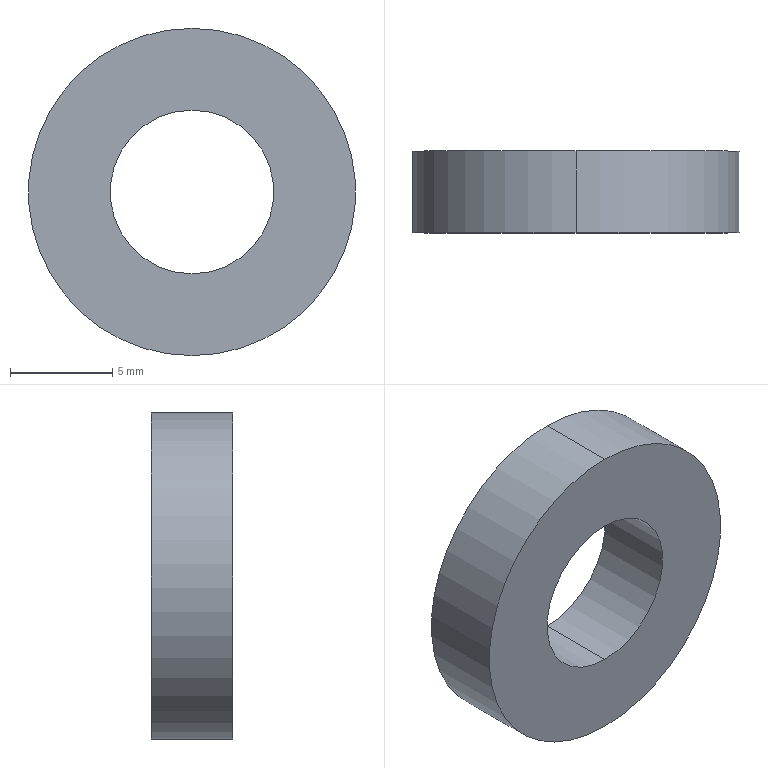Part | SolidWorks | features Revolution 1 | 1 solid | 6 faces | box 16 x 4 x 16 mm | volume 603.186 mm3 | cylinder 4 | plane 2 | commonest cylinder face diameters 8 x2 16 x2
STEP:
#1=CARTESIAN_POINT('',(0.,1.1,-8.));
#2=VERTEX_POINT('',#1);
#3=CARTESIAN_POINT('',(0.,1.1,8.));
#4=VERTEX_POINT('',#3);
#5=CARTESIAN_POINT('',(0.,1.1,0.));
#6=DIRECTION('',(0.,-1.,0.));
#7=DIRECTION('',(0.,0.,-1.));
#8=AXIS2_PLACEMENT_3D('',#5,#6,#7);
#9=CIRCLE('',#8,8.);
#10=EDGE_CURVE('',#2,#4,#9,.T.);
#11=ORIENTED_EDGE('',*,*,#10,.T.);
#12=CARTESIAN_POINT('',(0.,-2.9,8.));
#13=VERTEX_POINT('',#12);
#14=CARTESIAN_POINT('',(0.,0.,8.));
#15=DIRECTION('',(0.,-1.,0.));
#16=VECTOR('',#15,1000.);
#17=LINE('',#14,#16);
#18=EDGE_CURVE('',#4,#13,#17,.T.);
#19=ORIENTED_EDGE('',*,*,#18,.T.);
#20=CARTESIAN_POINT('',(0.,-2.9,-8.));
#21=VERTEX_POINT('',#20);
#22=CARTESIAN_POINT('',(0.,-2.9,0.));
#23=DIRECTION('',(0.,-1.,0.));
#24=DIRECTION('',(0.,0.,-1.));
#25=AXIS2_PLACEMENT_3D('',#22,#23,#24);
#26=CIRCLE('',#25,8.);
#27=EDGE_CURVE('',#21,#13,#26,.T.);
#28=ORIENTED_EDGE('',*,*,#27,.F.);
#29=CARTESIAN_POINT('',(0.,0.,-8.));
#30=DIRECTION('',(0.,-1.,0.));
#31=VECTOR('',#30,1000.);
#32=LINE('',#29,#31);
#33=EDGE_CURVE('',#2,#21,#32,.T.);
#34=ORIENTED_EDGE('',*,*,#33,.F.);
#35=EDGE_LOOP('',(#11,#19,#28,#34));
#36=FACE_OUTER_BOUND('',#35,.T.);
#37=CARTESIAN_POINT('',(0.,0.,0.));
#38=DIRECTION('',(0.,-1.,0.));
#39=DIRECTION('',(0.,0.,-1.));
#40=AXIS2_PLACEMENT_3D('',#37,#38,#39);
#41=CYLINDRICAL_SURFACE('',#40,8.);
#42=ADVANCED_FACE('',(#36),#41,.T.);
#43=CARTESIAN_POINT('',(0.,1.1,4.));
#44=VERTEX_POINT('',#43);
#45=CARTESIAN_POINT('',(0.,1.1,-4.));
#46=VERTEX_POINT('',#45);
#47=CARTESIAN_POINT('',(0.,1.1,0.));
#48=DIRECTION('',(0.,-1.,0.));
#49=DIRECTION('',(0.,0.,-1.));
#50=AXIS2_PLACEMENT_3D('',#47,#48,#49);
#51=CIRCLE('',#50,4.);
#52=EDGE_CURVE('',#44,#46,#51,.T.);
#53=ORIENTED_EDGE('',*,*,#52,.F.);
#54=CARTESIAN_POINT('',(0.,-2.9,4.));
#55=VERTEX_POINT('',#54);
#56=CARTESIAN_POINT('',(0.,0.,4.));
#57=DIRECTION('',(0.,-1.,0.));
#58=VECTOR('',#57,1000.);
#59=LINE('',#56,#58);
#60=EDGE_CURVE('',#44,#55,#59,.T.);
#61=ORIENTED_EDGE('',*,*,#60,.T.);
#62=CARTESIAN_POINT('',(0.,-2.9,-4.));
#63=VERTEX_POINT('',#62);
#64=CARTESIAN_POINT('',(0.,-2.9,0.));
#65=DIRECTION('',(0.,-1.,0.));
#66=DIRECTION('',(0.,0.,-1.));
#67=AXIS2_PLACEMENT_3D('',#64,#65,#66);
#68=CIRCLE('',#67,4.);
#69=EDGE_CURVE('',#55,#63,#68,.T.);
#70=ORIENTED_EDGE('',*,*,#69,.T.);
#71=CARTESIAN_POINT('',(0.,0.,-4.));
#72=DIRECTION('',(0.,-1.,0.));
#73=VECTOR('',#72,1000.);
#74=LINE('',#71,#73);
#75=EDGE_CURVE('',#46,#63,#74,.T.);
#76=ORIENTED_EDGE('',*,*,#75,.F.);
#77=EDGE_LOOP('',(#53,#61,#70,#76));
#78=FACE_OUTER_BOUND('',#77,.T.);
#79=CARTESIAN_POINT('',(0.,0.,0.));
#80=DIRECTION('',(0.,-1.,0.));
#81=DIRECTION('',(0.,0.,-1.));
#82=AXIS2_PLACEMENT_3D('',#79,#80,#81);
#83=CYLINDRICAL_SURFACE('',#82,4.);
#84=ADVANCED_FACE('',(#78),#83,.F.);
#85=ORIENTED_EDGE('',*,*,#60,.F.);
#86=CARTESIAN_POINT('',(0.,1.1,0.));
#87=DIRECTION('',(0.,-1.,0.));
#88=DIRECTION('',(0.,0.,-1.));
#89=AXIS2_PLACEMENT_3D('',#86,#87,#88);
#90=CIRCLE('',#89,4.);
#91=EDGE_CURVE('',#46,#44,#90,.T.);
#92=ORIENTED_EDGE('',*,*,#91,.F.);
#93=ORIENTED_EDGE('',*,*,#75,.T.);
#94=CARTESIAN_POINT('',(0.,-2.9,0.));
#95=DIRECTION('',(0.,-1.,0.));
#96=DIRECTION('',(0.,0.,-1.));
#97=AXIS2_PLACEMENT_3D('',#94,#95,#96);
#98=CIRCLE('',#97,4.);
#99=EDGE_CURVE('',#63,#55,#98,.T.);
#100=ORIENTED_EDGE('',*,*,#99,.T.);
#101=EDGE_LOOP('',(#85,#92,#93,#100));
#102=FACE_OUTER_BOUND('',#101,.T.);
#103=CARTESIAN_POINT('',(0.,0.,0.));
#104=DIRECTION('',(0.,-1.,0.));
#105=DIRECTION('',(0.,0.,-1.));
#106=AXIS2_PLACEMENT_3D('',#103,#104,#105);
#107=CYLINDRICAL_SURFACE('',#106,4.);
#108=ADVANCED_FACE('',(#102),#107,.F.);
#109=ORIENTED_EDGE('',*,*,#91,.T.);
#110=ORIENTED_EDGE('',*,*,#52,.T.);
#111=EDGE_LOOP('',(#109,#110));
#112=FACE_BOUND('',#111,.T.);
#113=ORIENTED_EDGE('',*,*,#10,.F.);
#114=CARTESIAN_POINT('',(0.,1.1,0.));
#115=DIRECTION('',(0.,-1.,0.));
#116=DIRECTION('',(0.,0.,-1.));
#117=AXIS2_PLACEMENT_3D('',#114,#115,#116);
#118=CIRCLE('',#117,8.);
#119=EDGE_CURVE('',#4,#2,#118,.T.);
#120=ORIENTED_EDGE('',*,*,#119,.F.);
#121=EDGE_LOOP('',(#113,#120));
#122=FACE_OUTER_BOUND('',#121,.T.);
#123=CARTESIAN_POINT('',(4.,1.1,0.));
#124=DIRECTION('',(0.,1.,0.));
#125=DIRECTION('',(0.,0.,1.));
#126=AXIS2_PLACEMENT_3D('',#123,#124,#125);
#127=PLANE('',#126);
#128=ADVANCED_FACE('',(#112,#122),#127,.T.);
#129=ORIENTED_EDGE('',*,*,#18,.F.);
#130=ORIENTED_EDGE('',*,*,#119,.T.);
#131=ORIENTED_EDGE('',*,*,#33,.T.);
#132=CARTESIAN_POINT('',(0.,-2.9,0.));
#133=DIRECTION('',(0.,-1.,0.));
#134=DIRECTION('',(0.,0.,-1.));
#135=AXIS2_PLACEMENT_3D('',#132,#133,#134);
#136=CIRCLE('',#135,8.);
#137=EDGE_CURVE('',#13,#21,#136,.T.);
#138=ORIENTED_EDGE('',*,*,#137,.F.);
#139=EDGE_LOOP('',(#129,#130,#131,#138));
#140=FACE_OUTER_BOUND('',#139,.T.);
#141=CARTESIAN_POINT('',(0.,0.,0.));
#142=DIRECTION('',(0.,-1.,0.));
#143=DIRECTION('',(0.,0.,-1.));
#144=AXIS2_PLACEMENT_3D('',#141,#142,#143);
#145=CYLINDRICAL_SURFACE('',#144,8.);
#146=ADVANCED_FACE('',(#140),#145,.T.);
#147=ORIENTED_EDGE('',*,*,#27,.T.);
#148=ORIENTED_EDGE('',*,*,#137,.T.);
#149=EDGE_LOOP('',(#147,#148));
#150=FACE_OUTER_BOUND('',#149,.T.);
#151=ORIENTED_EDGE('',*,*,#99,.F.);
#152=ORIENTED_EDGE('',*,*,#69,.F.);
#153=EDGE_LOOP('',(#151,#152));
#154=FACE_BOUND('',#153,.T.);
#155=CARTESIAN_POINT('',(8.,-2.9,0.));
#156=DIRECTION('',(0.,-1.,0.));
#157=DIRECTION('',(0.,0.,-1.));
#158=AXIS2_PLACEMENT_3D('',#155,#156,#157);
#159=PLANE('',#158);
#160=ADVANCED_FACE('',(#150,#154),#159,.T.);
#161=CLOSED_SHELL('',(#42,#84,#108,#128,#146,#160));
#162=MANIFOLD_SOLID_BREP('',#161);
#163=CARTESIAN_POINT('',(0.,0.,0.));
#164=DIRECTION('',(0.,0.,1.));
#165=DIRECTION('',(1.,0.,0.));
#166=AXIS2_PLACEMENT_3D('',#163,#164,#165);
#167=(LENGTH_UNIT()NAMED_UNIT(*)SI_UNIT(.MILLI.,.METRE.));
#168=UNCERTAINTY_MEASURE_WITH_UNIT(LENGTH_MEASURE(0.00001),#167,'','');
#169=(NAMED_UNIT(*)PLANE_ANGLE_UNIT()SI_UNIT($,.RADIAN.));
#170=(NAMED_UNIT(*)SI_UNIT($,.STERADIAN.)SOLID_ANGLE_UNIT());
#171=(GEOMETRIC_REPRESENTATION_CONTEXT(3)GLOBAL_UNCERTAINTY_ASSIGNED_CONTEXT((#168))GLOBAL_UNIT_ASSIGNED_CONTEXT((#167,#169,#170))REPRESENTATION_CONTEXT('',''));
#172=ADVANCED_BREP_SHAPE_REPRESENTATION('',(#162,#166),#171);